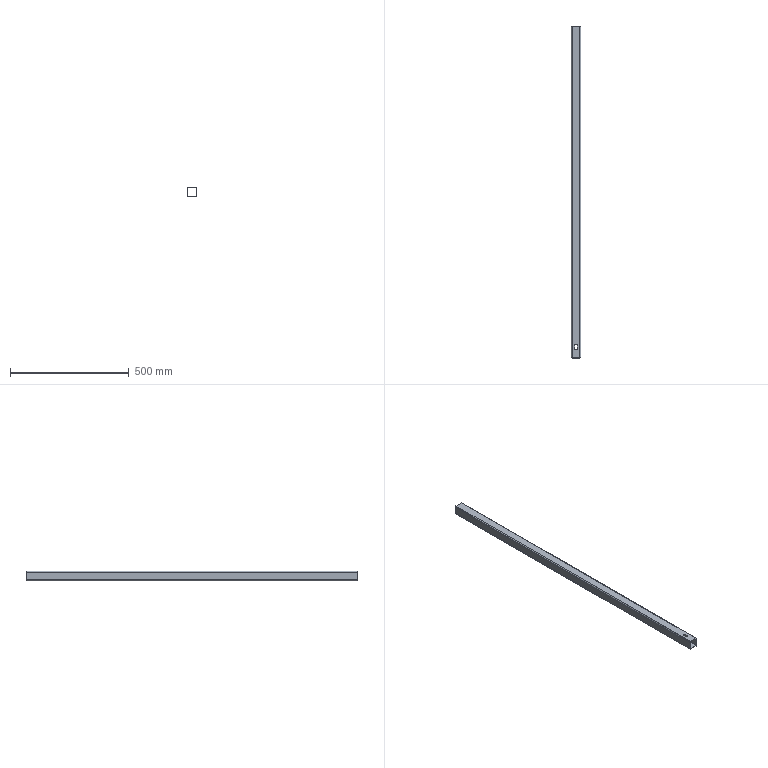Part | STEP file | E3-护栏立柱8-2主体_Default<As Machined> | 1 solid | 26 faces | box 40 x 1400 x 40 mm | volume 410246 mm3 | plane 14 | cylinder 12 | commonest cylinder face diameters 4 x4 8 x4 12 x4